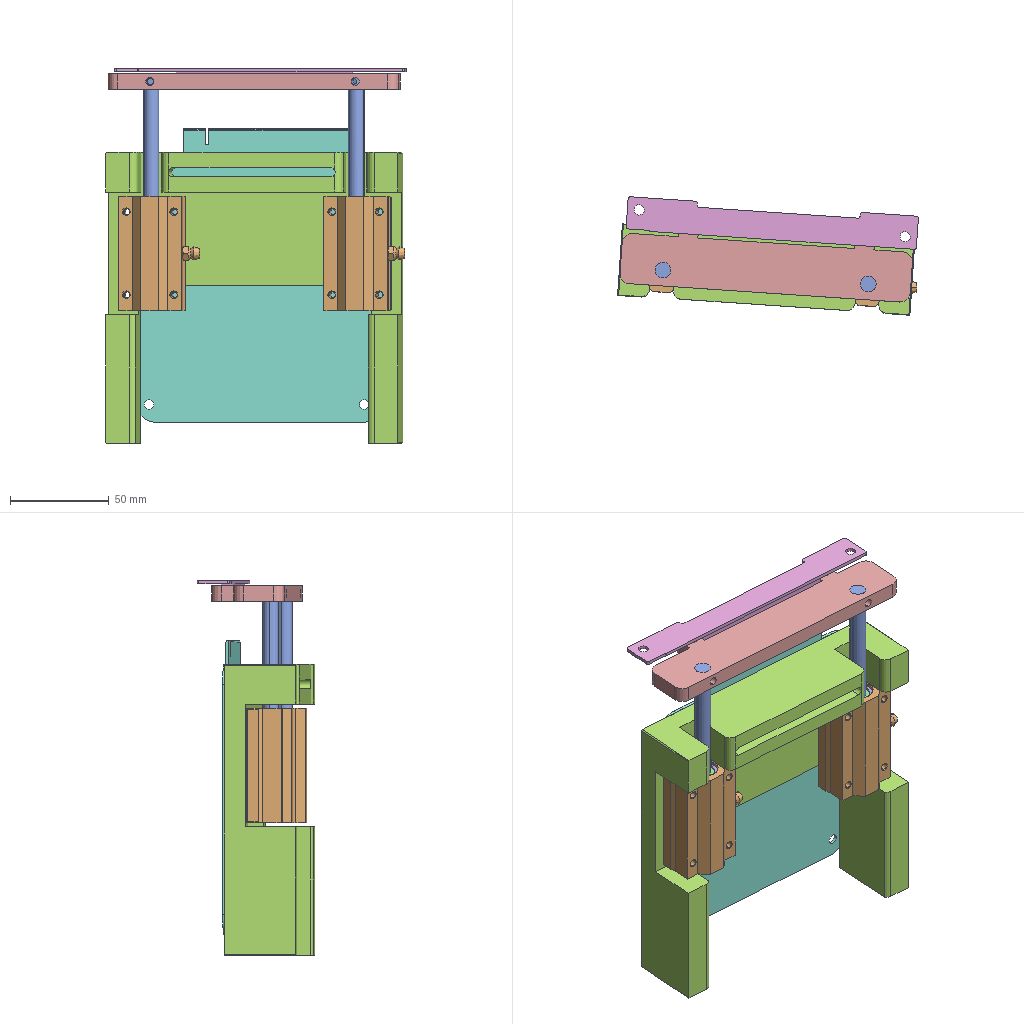Assembly | SolidWorks | 10 different items | 20 placed | box 152 x 60 x 189 mm
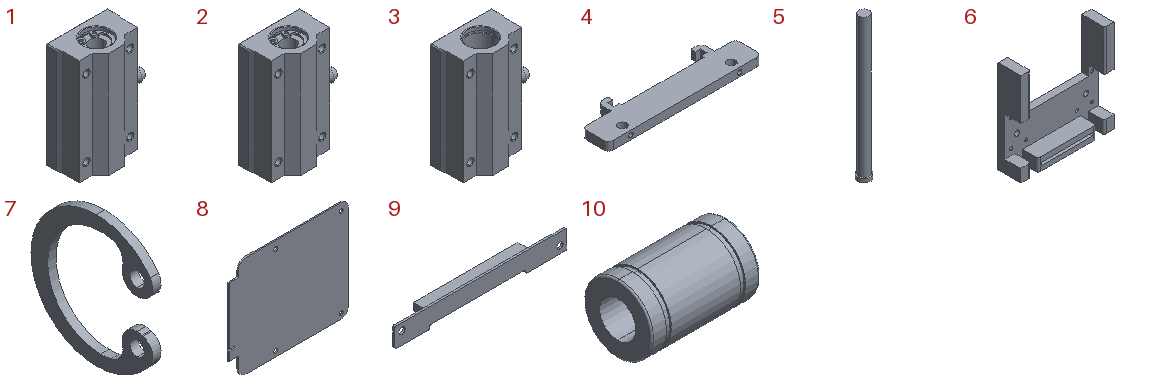Parts list (item | name | quantity | parent item | size | volume | features):
1 | (subassembly) | x2 | in 2 | 41.5 x 22 x 58 mm | 31868 mm3 | -
2 | (subassembly) | x2 | - | 41.5 x 22 x 58 mm | 31868 mm3 | -
3 | - | x2 | in 1 | 41.5 x 22 x 58 mm | 25731 mm3 | features MBimport 1
4 | - | x1 | - | 147 x 38.4 x 8 mm | 30280 mm3 | features ICE 5, Fillet 3, Chamfer 1, Extrusion 1, HoleWzd 1, MirrorPattern 1
5 | - | x2 | - | 10 x 10 x 113 mm | 5731 mm3 | features Extrusion 1, HoleWzd 1, ICE 1
6 | - | x1 | - | 148 x 36 x 147 mm | 224045 mm3 | features ICE 6, HoleWzd 2, Chamfer 1, Extrusion 1, Fillet 1
7 | - | x4 | in 1 | 1 x 14.572 x 15.7 mm | 72.207 mm3 | features MBimport 1
8 | - | x1 | - | 148.4 x 1.6 x 125 mm | 28585 mm3 | features Chamfer 2, Fillet 2, ICE 2, Extrusion 1, HoleWzd 1
9 | - | x1 | - | 147 x 10.5 x 16.8 mm | 7195 mm3 | features ICE 3, Extrusion 1, MoveFace 1
10 | - | x4 | in 1 | 24 x 15 x 15 mm | 2996 mm3 | features MBimport 1
Mates (type | each side: item.copy, entity, surface, feature):
Concentric | 4.1 face cylinder Cut-Extrude1 | 5.1 face cylinder Boss-Extrude1
Concentric | 4.1 face cylinder Cut-Extrude1 | 5.2 face cylinder Boss-Extrude1
Coincident | 4.1 face plane Boss-Extrude4 | 9.1 face plane Boss-Extrude3
Coincident | 4.1 face plane Boss-Extrude2 | 9.1 face plane Cut-Extrude1
Coincident | 4.1 face plane Boss-Extrude1 | 9.1 face plane Boss-Extrude3
Coincident | 6.1 face plane Boss-Extrude1 | 8.1 face plane Boss-Extrude1
Coincident | 4.1 face plane Boss-Extrude1 | 5.2 face plane Boss-Extrude1
Coincident | 4.1 face plane Boss-Extrude1 | 5.1 face plane Boss-Extrude1
Concentric | 5.2 face cylinder Boss-Extrude1 | 10.1 face cylinder E-LBHNW8-P.stp<1>
Concentric | 5.1 face cylinder Boss-Extrude1 | 10.2 face cylinder E-LBHNW8-P.stp<1>
Width | 6.1 face plane Cut-Extrude2 | 6.1 face plane Cut-Extrude2 | 3.1 face plane E-LBHNW8-P.stp<1> | 3.1 face plane E-LBHNW8-P.stp<1>
Parallel | 4.1 face plane Boss-Extrude1 | 3.2 face plane E-LBHNW8-P.stp<1>
Parallel | 4.1 face plane Boss-Extrude1 | 3.1 face plane E-LBHNW8-P.stp<1>
Coincident | 6.1 face plane Cut-Extrude1 | 3.1 face plane E-LBHNW8-P.stp<1>
Concentric | 6.1 face cylinder CBORE for M4 Slotted cheese head screws1 | 3.1 face cylinder E-LBHNW8-P.stp<1>
Concentric | 6.1 face cylinder CBORE for M4 Slotted cheese head screws1 | 3.2 face cylinder E-LBHNW8-P.stp<1>